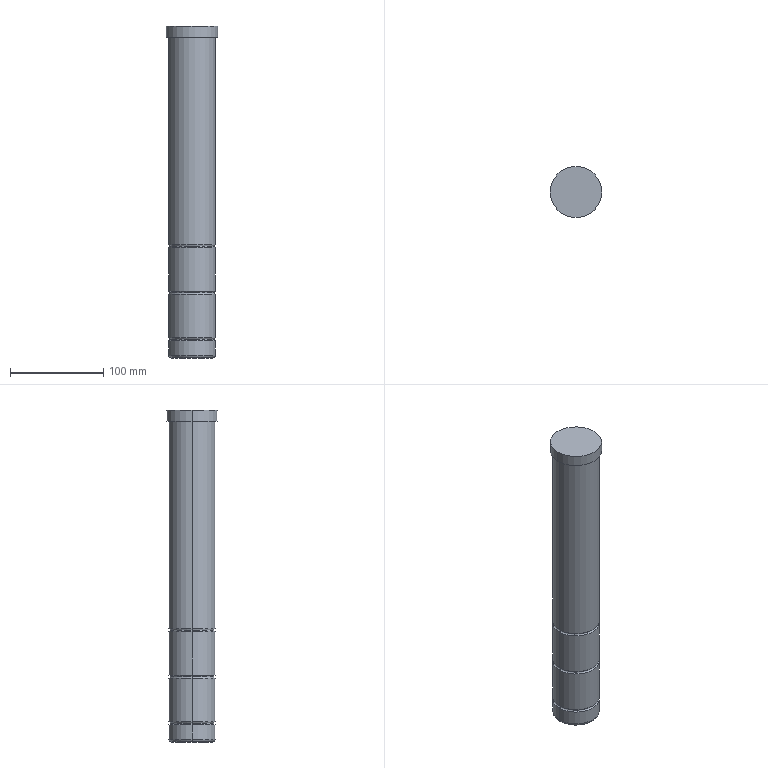Part | Creo | 1 solid | 29 faces | box 55 x 55 x 356 mm | volume 702034 mm3 | torus 16 | cylinder 10 | plane 3 | commonest cylinder face diameters 50 x8 55 x2
STEP:
#1=CARTESIAN_POINT('',(-272.,297.,-127.));
#2=VERTEX_POINT('',#1);
#3=CARTESIAN_POINT('',(-222.,297.,-127.));
#4=VERTEX_POINT('',#3);
#5=CARTESIAN_POINT('',(-247.,297.,-127.));
#6=DIRECTION('',(0.,0.,1.));
#7=DIRECTION('',(-1.,0.,0.));
#8=AXIS2_PLACEMENT_3D('',#5,#6,#7);
#9=CIRCLE('',#8,25.);
#10=EDGE_CURVE('',#2,#4,#9,.T.);
#11=ORIENTED_EDGE('',*,*,#10,.T.);
#12=CARTESIAN_POINT('',(-222.,297.,-142.5));
#13=VERTEX_POINT('',#12);
#14=CARTESIAN_POINT('',(-222.,297.,-127.));
#15=DIRECTION('',(0.,0.,-1.));
#16=VECTOR('',#15,15.5);
#17=LINE('',#14,#16);
#18=EDGE_CURVE('',#4,#13,#17,.T.);
#19=ORIENTED_EDGE('',*,*,#18,.T.);
#20=CARTESIAN_POINT('',(-272.,297.,-142.5));
#21=VERTEX_POINT('',#20);
#22=CARTESIAN_POINT('',(-247.,297.,-142.5));
#23=DIRECTION('',(0.,0.,-1.));
#24=DIRECTION('',(1.,0.,0.));
#25=AXIS2_PLACEMENT_3D('',#22,#23,#24);
#26=CIRCLE('',#25,25.);
#27=EDGE_CURVE('',#13,#21,#26,.T.);
#28=ORIENTED_EDGE('',*,*,#27,.T.);
#29=CARTESIAN_POINT('',(-272.,297.,-127.));
#30=DIRECTION('',(0.,0.,-1.));
#31=VECTOR('',#30,15.5);
#32=LINE('',#29,#31);
#33=EDGE_CURVE('',#2,#21,#32,.T.);
#34=ORIENTED_EDGE('',*,*,#33,.F.);
#35=EDGE_LOOP('',(#11,#19,#28,#34));
#36=FACE_OUTER_BOUND('',#35,.F.);
#37=CARTESIAN_POINT('',(-247.,297.,150.5));
#38=DIRECTION('',(0.,0.,-1.));
#39=DIRECTION('',(1.,0.,0.));
#40=AXIS2_PLACEMENT_3D('',#37,#38,#39);
#41=CYLINDRICAL_SURFACE('',#40,25.);
#42=ADVANCED_FACE('',(#36),#41,.T.);
#43=ORIENTED_EDGE('',*,*,#10,.F.);
#44=CARTESIAN_POINT('',(-270.5,297.,-125.5));
#45=VERTEX_POINT('',#44);
#46=CARTESIAN_POINT('',(-272.,297.,-125.5));
#47=DIRECTION('',(0.,-1.,0.));
#48=DIRECTION('',(0.,0.,-1.));
#49=AXIS2_PLACEMENT_3D('',#46,#47,#48);
#50=CIRCLE('',#49,1.5);
#51=EDGE_CURVE('',#2,#45,#50,.T.);
#52=ORIENTED_EDGE('',*,*,#51,.T.);
#53=CARTESIAN_POINT('',(-223.5,297.,-125.5));
#54=VERTEX_POINT('',#53);
#55=CARTESIAN_POINT('',(-247.,297.,-125.5));
#56=DIRECTION('',(0.,0.,-1.));
#57=DIRECTION('',(1.,0.,0.));
#58=AXIS2_PLACEMENT_3D('',#55,#56,#57);
#59=CIRCLE('',#58,23.5);
#60=EDGE_CURVE('',#54,#45,#59,.T.);
#61=ORIENTED_EDGE('',*,*,#60,.F.);
#62=CARTESIAN_POINT('',(-222.,297.,-125.5));
#63=DIRECTION('',(0.,1.,0.));
#64=DIRECTION('',(0.,0.,-1.));
#65=AXIS2_PLACEMENT_3D('',#62,#63,#64);
#66=CIRCLE('',#65,1.5);
#67=EDGE_CURVE('',#4,#54,#66,.T.);
#68=ORIENTED_EDGE('',*,*,#67,.F.);
#69=EDGE_LOOP('',(#43,#52,#61,#68));
#70=FACE_OUTER_BOUND('',#69,.F.);
#71=CARTESIAN_POINT('',(-247.,297.,-125.5));
#72=DIRECTION('',(0.,0.,-1.));
#73=DIRECTION('',(1.,0.,0.));
#74=AXIS2_PLACEMENT_3D('',#71,#72,#73);
#75=TOROIDAL_SURFACE('',#74,25.,1.5);
#76=ADVANCED_FACE('',(#70),#75,.F.);
#77=CARTESIAN_POINT('',(-247.,297.,-127.));
#78=DIRECTION('',(0.,0.,1.));
#79=DIRECTION('',(1.,0.,0.));
#80=AXIS2_PLACEMENT_3D('',#77,#78,#79);
#81=CIRCLE('',#80,25.);
#82=EDGE_CURVE('',#4,#2,#81,.T.);
#83=ORIENTED_EDGE('',*,*,#82,.F.);
#84=ORIENTED_EDGE('',*,*,#67,.T.);
#85=CARTESIAN_POINT('',(-247.,297.,-125.5));
#86=DIRECTION('',(0.,0.,-1.));
#87=DIRECTION('',(-1.,0.,0.));
#88=AXIS2_PLACEMENT_3D('',#85,#86,#87);
#89=CIRCLE('',#88,23.5);
#90=EDGE_CURVE('',#45,#54,#89,.T.);
#91=ORIENTED_EDGE('',*,*,#90,.F.);
#92=ORIENTED_EDGE('',*,*,#51,.F.);
#93=EDGE_LOOP('',(#83,#84,#91,#92));
#94=FACE_OUTER_BOUND('',#93,.F.);
#95=CARTESIAN_POINT('',(-247.,297.,-125.5));
#96=DIRECTION('',(0.,0.,-1.));
#97=DIRECTION('',(1.,0.,0.));
#98=AXIS2_PLACEMENT_3D('',#95,#96,#97);
#99=TOROIDAL_SURFACE('',#98,25.,1.5);
#100=ADVANCED_FACE('',(#94),#99,.F.);
#101=ORIENTED_EDGE('',*,*,#82,.T.);
#102=ORIENTED_EDGE('',*,*,#33,.T.);
#103=CARTESIAN_POINT('',(-247.,297.,-142.5));
#104=DIRECTION('',(0.,0.,-1.));
#105=DIRECTION('',(-1.,0.,0.));
#106=AXIS2_PLACEMENT_3D('',#103,#104,#105);
#107=CIRCLE('',#106,25.);
#108=EDGE_CURVE('',#21,#13,#107,.T.);
#109=ORIENTED_EDGE('',*,*,#108,.T.);
#110=ORIENTED_EDGE('',*,*,#18,.F.);
#111=EDGE_LOOP('',(#101,#102,#109,#110));
#112=FACE_OUTER_BOUND('',#111,.F.);
#113=CARTESIAN_POINT('',(-247.,297.,150.5));
#114=DIRECTION('',(0.,0.,-1.));
#115=DIRECTION('',(1.,0.,0.));
#116=AXIS2_PLACEMENT_3D('',#113,#114,#115);
#117=CYLINDRICAL_SURFACE('',#116,25.);
#118=ADVANCED_FACE('',(#112),#117,.T.);
#119=ORIENTED_EDGE('',*,*,#108,.F.);
#120=CARTESIAN_POINT('',(-271.121,297.,-144.621));
#121=VERTEX_POINT('',#120);
#122=CARTESIAN_POINT('',(-269.,297.,-142.5));
#123=DIRECTION('',(0.,-1.,0.));
#124=DIRECTION('',(-1.,0.,0.));
#125=AXIS2_PLACEMENT_3D('',#122,#123,#124);
#126=CIRCLE('',#125,3.);
#127=EDGE_CURVE('',#21,#121,#126,.T.);
#128=ORIENTED_EDGE('',*,*,#127,.T.);
#129=CARTESIAN_POINT('',(-222.879,297.,-144.621));
#130=VERTEX_POINT('',#129);
#131=CARTESIAN_POINT('',(-247.,297.,-144.621));
#132=DIRECTION('',(0.,0.,-1.));
#133=DIRECTION('',(-1.,0.,0.));
#134=AXIS2_PLACEMENT_3D('',#131,#132,#133);
#135=CIRCLE('',#134,24.121);
#136=EDGE_CURVE('',#121,#130,#135,.T.);
#137=ORIENTED_EDGE('',*,*,#136,.T.);
#138=CARTESIAN_POINT('',(-225.,297.,-142.5));
#139=DIRECTION('',(0.,1.,0.));
#140=DIRECTION('',(1.,0.,0.));
#141=AXIS2_PLACEMENT_3D('',#138,#139,#140);
#142=CIRCLE('',#141,3.);
#143=EDGE_CURVE('',#13,#130,#142,.T.);
#144=ORIENTED_EDGE('',*,*,#143,.F.);
#145=EDGE_LOOP('',(#119,#128,#137,#144));
#146=FACE_OUTER_BOUND('',#145,.F.);
#147=CARTESIAN_POINT('',(-247.,297.,-142.5));
#148=DIRECTION('',(0.,0.,-1.));
#149=DIRECTION('',(1.,0.,0.));
#150=AXIS2_PLACEMENT_3D('',#147,#148,#149);
#151=TOROIDAL_SURFACE('',#150,22.,3.);
#152=ADVANCED_FACE('',(#146),#151,.T.);
#153=ORIENTED_EDGE('',*,*,#27,.F.);
#154=ORIENTED_EDGE('',*,*,#143,.T.);
#155=CARTESIAN_POINT('',(-247.,297.,-144.621));
#156=DIRECTION('',(0.,0.,-1.));
#157=DIRECTION('',(1.,0.,0.));
#158=AXIS2_PLACEMENT_3D('',#155,#156,#157);
#159=CIRCLE('',#158,24.121);
#160=EDGE_CURVE('',#130,#121,#159,.T.);
#161=ORIENTED_EDGE('',*,*,#160,.T.);
#162=ORIENTED_EDGE('',*,*,#127,.F.);
#163=EDGE_LOOP('',(#153,#154,#161,#162));
#164=FACE_OUTER_BOUND('',#163,.F.);
#165=CARTESIAN_POINT('',(-247.,297.,-142.5));
#166=DIRECTION('',(0.,0.,-1.));
#167=DIRECTION('',(1.,0.,0.));
#168=AXIS2_PLACEMENT_3D('',#165,#166,#167);
#169=TOROIDAL_SURFACE('',#168,22.,3.);
#170=ADVANCED_FACE('',(#164),#169,.T.);
#171=CARTESIAN_POINT('',(-225.,297.,-145.5));
#172=VERTEX_POINT('',#171);
#173=CARTESIAN_POINT('',(-269.,297.,-145.5));
#174=VERTEX_POINT('',#173);
#175=CARTESIAN_POINT('',(-247.,297.,-145.5));
#176=DIRECTION('',(0.,0.,-1.));
#177=DIRECTION('',(1.,0.,0.));
#178=AXIS2_PLACEMENT_3D('',#175,#176,#177);
#179=CIRCLE('',#178,22.);
#180=EDGE_CURVE('',#172,#174,#179,.T.);
#181=ORIENTED_EDGE('',*,*,#180,.T.);
#182=CARTESIAN_POINT('',(-269.,297.,-142.5));
#183=DIRECTION('',(0.,-1.,0.));
#184=DIRECTION('',(-0.7071,0.,-0.7071));
#185=AXIS2_PLACEMENT_3D('',#182,#183,#184);
#186=CIRCLE('',#185,3.);
#187=EDGE_CURVE('',#121,#174,#186,.T.);
#188=ORIENTED_EDGE('',*,*,#187,.F.);
#189=ORIENTED_EDGE('',*,*,#160,.F.);
#190=CARTESIAN_POINT('',(-225.,297.,-142.5));
#191=DIRECTION('',(0.,1.,0.));
#192=DIRECTION('',(0.7071,0.,-0.7071));
#193=AXIS2_PLACEMENT_3D('',#190,#191,#192);
#194=CIRCLE('',#193,3.);
#195=EDGE_CURVE('',#130,#172,#194,.T.);
#196=ORIENTED_EDGE('',*,*,#195,.T.);
#197=EDGE_LOOP('',(#181,#188,#189,#196));
#198=FACE_OUTER_BOUND('',#197,.F.);
#199=CARTESIAN_POINT('',(-247.,297.,-142.5));
#200=DIRECTION('',(0.,0.,-1.));
#201=DIRECTION('',(1.,0.,0.));
#202=AXIS2_PLACEMENT_3D('',#199,#200,#201);
#203=TOROIDAL_SURFACE('',#202,22.,3.);
#204=ADVANCED_FACE('',(#198),#203,.T.);
#205=ORIENTED_EDGE('',*,*,#180,.F.);
#206=CARTESIAN_POINT('',(-247.,297.,-145.5));
#207=DIRECTION('',(0.,0.,-1.));
#208=DIRECTION('',(-1.,0.,0.));
#209=AXIS2_PLACEMENT_3D('',#206,#207,#208);
#210=CIRCLE('',#209,22.);
#211=EDGE_CURVE('',#174,#172,#210,.T.);
#212=ORIENTED_EDGE('',*,*,#211,.F.);
#213=EDGE_LOOP('',(#205,#212));
#214=FACE_OUTER_BOUND('',#213,.F.);
#215=CARTESIAN_POINT('',(-247.,297.,-145.5));
#216=DIRECTION('',(0.,0.,-1.));
#217=DIRECTION('',(1.,0.,0.));
#218=AXIS2_PLACEMENT_3D('',#215,#216,#217);
#219=PLANE('',#218);
#220=ADVANCED_FACE('',(#214),#219,.T.);
#221=ORIENTED_EDGE('',*,*,#211,.T.);
#222=ORIENTED_EDGE('',*,*,#195,.F.);
#223=ORIENTED_EDGE('',*,*,#136,.F.);
#224=ORIENTED_EDGE('',*,*,#187,.T.);
#225=EDGE_LOOP('',(#221,#222,#223,#224));
#226=FACE_OUTER_BOUND('',#225,.F.);
#227=CARTESIAN_POINT('',(-247.,297.,-142.5));
#228=DIRECTION('',(0.,0.,-1.));
#229=DIRECTION('',(1.,0.,0.));
#230=AXIS2_PLACEMENT_3D('',#227,#228,#229);
#231=TOROIDAL_SURFACE('',#230,22.,3.);
#232=ADVANCED_FACE('',(#226),#231,.T.);
#233=CARTESIAN_POINT('',(-272.,297.,-124.));
#234=VERTEX_POINT('',#233);
#235=CARTESIAN_POINT('',(-222.,297.,-124.));
#236=VERTEX_POINT('',#235);
#237=CARTESIAN_POINT('',(-247.,297.,-124.));
#238=DIRECTION('',(0.,0.,-1.));
#239=DIRECTION('',(-1.,0.,0.));
#240=AXIS2_PLACEMENT_3D('',#237,#238,#239);
#241=CIRCLE('',#240,25.);
#242=EDGE_CURVE('',#234,#236,#241,.T.);
#243=ORIENTED_EDGE('',*,*,#242,.F.);
#244=CARTESIAN_POINT('',(-272.,297.,-125.5));
#245=DIRECTION('',(0.,-1.,0.));
#246=DIRECTION('',(1.,0.,0.));
#247=AXIS2_PLACEMENT_3D('',#244,#245,#246);
#248=CIRCLE('',#247,1.5);
#249=EDGE_CURVE('',#45,#234,#248,.T.);
#250=ORIENTED_EDGE('',*,*,#249,.F.);
#251=ORIENTED_EDGE('',*,*,#90,.T.);
#252=CARTESIAN_POINT('',(-222.,297.,-125.5));
#253=DIRECTION('',(0.,1.,0.));
#254=DIRECTION('',(-1.,0.,0.));
#255=AXIS2_PLACEMENT_3D('',#252,#253,#254);
#256=CIRCLE('',#255,1.5);
#257=EDGE_CURVE('',#54,#236,#256,.T.);
#258=ORIENTED_EDGE('',*,*,#257,.T.);
#259=EDGE_LOOP('',(#243,#250,#251,#258));
#260=FACE_OUTER_BOUND('',#259,.F.);
#261=CARTESIAN_POINT('',(-247.,297.,-125.5));
#262=DIRECTION('',(0.,0.,-1.));
#263=DIRECTION('',(1.,0.,0.));
#264=AXIS2_PLACEMENT_3D('',#261,#262,#263);
#265=TOROIDAL_SURFACE('',#264,25.,1.5);
#266=ADVANCED_FACE('',(#260),#265,.F.);
#267=ORIENTED_EDGE('',*,*,#242,.T.);
#268=CARTESIAN_POINT('',(-222.,297.,-77.));
#269=VERTEX_POINT('',#268);
#270=CARTESIAN_POINT('',(-222.,297.,-77.));
#271=DIRECTION('',(0.,0.,-1.));
#272=VECTOR('',#271,47.);
#273=LINE('',#270,#272);
#274=EDGE_CURVE('',#269,#236,#273,.T.);
#275=ORIENTED_EDGE('',*,*,#274,.F.);
#276=CARTESIAN_POINT('',(-272.,297.,-77.));
#277=VERTEX_POINT('',#276);
#278=CARTESIAN_POINT('',(-247.,297.,-77.));
#279=DIRECTION('',(0.,0.,1.));
#280=DIRECTION('',(1.,0.,0.));
#281=AXIS2_PLACEMENT_3D('',#278,#279,#280);
#282=CIRCLE('',#281,25.);
#283=EDGE_CURVE('',#269,#277,#282,.T.);
#284=ORIENTED_EDGE('',*,*,#283,.T.);
#285=CARTESIAN_POINT('',(-272.,297.,-77.));
#286=DIRECTION('',(0.,0.,-1.));
#287=VECTOR('',#286,47.);
#288=LINE('',#285,#287);
#289=EDGE_CURVE('',#277,#234,#288,.T.);
#290=ORIENTED_EDGE('',*,*,#289,.T.);
#291=EDGE_LOOP('',(#267,#275,#284,#290));
#292=FACE_OUTER_BOUND('',#291,.F.);
#293=CARTESIAN_POINT('',(-247.,297.,150.5));
#294=DIRECTION('',(0.,0.,-1.));
#295=DIRECTION('',(1.,0.,0.));
#296=AXIS2_PLACEMENT_3D('',#293,#294,#295);
#297=CYLINDRICAL_SURFACE('',#296,25.);
#298=ADVANCED_FACE('',(#292),#297,.T.);
#299=CARTESIAN_POINT('',(-247.,297.,-124.));
#300=DIRECTION('',(0.,0.,-1.));
#301=DIRECTION('',(1.,0.,0.));
#302=AXIS2_PLACEMENT_3D('',#299,#300,#301);
#303=CIRCLE('',#302,25.);
#304=EDGE_CURVE('',#236,#234,#303,.T.);
#305=ORIENTED_EDGE('',*,*,#304,.T.);
#306=ORIENTED_EDGE('',*,*,#289,.F.);
#307=CARTESIAN_POINT('',(-247.,297.,-77.));
#308=DIRECTION('',(0.,0.,1.));
#309=DIRECTION('',(-1.,0.,0.));
#310=AXIS2_PLACEMENT_3D('',#307,#308,#309);
#311=CIRCLE('',#310,25.);
#312=EDGE_CURVE('',#277,#269,#311,.T.);
#313=ORIENTED_EDGE('',*,*,#312,.T.);
#314=ORIENTED_EDGE('',*,*,#274,.T.);
#315=EDGE_LOOP('',(#305,#306,#313,#314));
#316=FACE_OUTER_BOUND('',#315,.F.);
#317=CARTESIAN_POINT('',(-247.,297.,150.5));
#318=DIRECTION('',(0.,0.,-1.));
#319=DIRECTION('',(1.,0.,0.));
#320=AXIS2_PLACEMENT_3D('',#317,#318,#319);
#321=CYLINDRICAL_SURFACE('',#320,25.);
#322=ADVANCED_FACE('',(#316),#321,.T.);
#323=ORIENTED_EDGE('',*,*,#304,.F.);
#324=ORIENTED_EDGE('',*,*,#257,.F.);
#325=ORIENTED_EDGE('',*,*,#60,.T.);
#326=ORIENTED_EDGE('',*,*,#249,.T.);
#327=EDGE_LOOP('',(#323,#324,#325,#326));
#328=FACE_OUTER_BOUND('',#327,.F.);
#329=CARTESIAN_POINT('',(-247.,297.,-125.5));
#330=DIRECTION('',(0.,0.,-1.));
#331=DIRECTION('',(1.,0.,0.));
#332=AXIS2_PLACEMENT_3D('',#329,#330,#331);
#333=TOROIDAL_SURFACE('',#332,25.,1.5);
#334=ADVANCED_FACE('',(#328),#333,.F.);
#335=ORIENTED_EDGE('',*,*,#312,.F.);
#336=CARTESIAN_POINT('',(-270.5,297.,-75.5));
#337=VERTEX_POINT('',#336);
#338=CARTESIAN_POINT('',(-272.,297.,-75.5));
#339=DIRECTION('',(0.,-1.,0.));
#340=DIRECTION('',(0.,0.,-1.));
#341=AXIS2_PLACEMENT_3D('',#338,#339,#340);
#342=CIRCLE('',#341,1.5);
#343=EDGE_CURVE('',#277,#337,#342,.T.);
#344=ORIENTED_EDGE('',*,*,#343,.T.);
#345=CARTESIAN_POINT('',(-223.5,297.,-75.5));
#346=VERTEX_POINT('',#345);
#347=CARTESIAN_POINT('',(-247.,297.,-75.5));
#348=DIRECTION('',(0.,0.,-1.));
#349=DIRECTION('',(1.,0.,0.));
#350=AXIS2_PLACEMENT_3D('',#347,#348,#349);
#351=CIRCLE('',#350,23.5);
#352=EDGE_CURVE('',#346,#337,#351,.T.);
#353=ORIENTED_EDGE('',*,*,#352,.F.);
#354=CARTESIAN_POINT('',(-222.,297.,-75.5));
#355=DIRECTION('',(0.,1.,0.));
#356=DIRECTION('',(0.,0.,-1.));
#357=AXIS2_PLACEMENT_3D('',#354,#355,#356);
#358=CIRCLE('',#357,1.5);
#359=EDGE_CURVE('',#269,#346,#358,.T.);
#360=ORIENTED_EDGE('',*,*,#359,.F.);
#361=EDGE_LOOP('',(#335,#344,#353,#360));
#362=FACE_OUTER_BOUND('',#361,.F.);
#363=CARTESIAN_POINT('',(-247.,297.,-75.5));
#364=DIRECTION('',(0.,0.,-1.));
#365=DIRECTION('',(1.,0.,0.));
#366=AXIS2_PLACEMENT_3D('',#363,#364,#365);
#367=TOROIDAL_SURFACE('',#366,25.,1.5);
#368=ADVANCED_FACE('',(#362),#367,.F.);
#369=ORIENTED_EDGE('',*,*,#283,.F.);
#370=ORIENTED_EDGE('',*,*,#359,.T.);
#371=CARTESIAN_POINT('',(-247.,297.,-75.5));
#372=DIRECTION('',(0.,0.,-1.));
#373=DIRECTION('',(-1.,0.,0.));
#374=AXIS2_PLACEMENT_3D('',#371,#372,#373);
#375=CIRCLE('',#374,23.5);
#376=EDGE_CURVE('',#337,#346,#375,.T.);
#377=ORIENTED_EDGE('',*,*,#376,.F.);
#378=ORIENTED_EDGE('',*,*,#343,.F.);
#379=EDGE_LOOP('',(#369,#370,#377,#378));
#380=FACE_OUTER_BOUND('',#379,.F.);
#381=CARTESIAN_POINT('',(-247.,297.,-75.5));
#382=DIRECTION('',(0.,0.,-1.));
#383=DIRECTION('',(1.,0.,0.));
#384=AXIS2_PLACEMENT_3D('',#381,#382,#383);
#385=TOROIDAL_SURFACE('',#384,25.,1.5);
#386=ADVANCED_FACE('',(#380),#385,.F.);
#387=CARTESIAN_POINT('',(-272.,297.,-74.));
#388=VERTEX_POINT('',#387);
#389=CARTESIAN_POINT('',(-222.,297.,-74.));
#390=VERTEX_POINT('',#389);
#391=CARTESIAN_POINT('',(-247.,297.,-74.));
#392=DIRECTION('',(0.,0.,-1.));
#393=DIRECTION('',(-1.,0.,0.));
#394=AXIS2_PLACEMENT_3D('',#391,#392,#393);
#395=CIRCLE('',#394,25.);
#396=EDGE_CURVE('',#388,#390,#395,.T.);
#397=ORIENTED_EDGE('',*,*,#396,.F.);
#398=CARTESIAN_POINT('',(-272.,297.,-75.5));
#399=DIRECTION('',(0.,-1.,0.));
#400=DIRECTION('',(1.,0.,0.));
#401=AXIS2_PLACEMENT_3D('',#398,#399,#400);
#402=CIRCLE('',#401,1.5);
#403=EDGE_CURVE('',#337,#388,#402,.T.);
#404=ORIENTED_EDGE('',*,*,#403,.F.);
#405=ORIENTED_EDGE('',*,*,#376,.T.);
#406=CARTESIAN_POINT('',(-222.,297.,-75.5));
#407=DIRECTION('',(0.,1.,0.));
#408=DIRECTION('',(-1.,0.,0.));
#409=AXIS2_PLACEMENT_3D('',#406,#407,#408);
#410=CIRCLE('',#409,1.5);
#411=EDGE_CURVE('',#346,#390,#410,.T.);
#412=ORIENTED_EDGE('',*,*,#411,.T.);
#413=EDGE_LOOP('',(#397,#404,#405,#412));
#414=FACE_OUTER_BOUND('',#413,.F.);
#415=CARTESIAN_POINT('',(-247.,297.,-75.5));
#416=DIRECTION('',(0.,0.,-1.));
#417=DIRECTION('',(1.,0.,0.));
#418=AXIS2_PLACEMENT_3D('',#415,#416,#417);
#419=TOROIDAL_SURFACE('',#418,25.,1.5);
#420=ADVANCED_FACE('',(#414),#419,.F.);
#421=ORIENTED_EDGE('',*,*,#396,.T.);
#422=CARTESIAN_POINT('',(-222.,297.,-27.));
#423=VERTEX_POINT('',#422);
#424=CARTESIAN_POINT('',(-222.,297.,-27.));
#425=DIRECTION('',(0.,0.,-1.));
#426=VECTOR('',#425,47.);
#427=LINE('',#424,#426);
#428=EDGE_CURVE('',#423,#390,#427,.T.);
#429=ORIENTED_EDGE('',*,*,#428,.F.);
#430=CARTESIAN_POINT('',(-272.,297.,-27.));
#431=VERTEX_POINT('',#430);
#432=CARTESIAN_POINT('',(-247.,297.,-27.));
#433=DIRECTION('',(0.,0.,1.));
#434=DIRECTION('',(1.,0.,0.));
#435=AXIS2_PLACEMENT_3D('',#432,#433,#434);
#436=CIRCLE('',#435,25.);
#437=EDGE_CURVE('',#423,#431,#436,.T.);
#438=ORIENTED_EDGE('',*,*,#437,.T.);
#439=CARTESIAN_POINT('',(-272.,297.,-27.));
#440=DIRECTION('',(0.,0.,-1.));
#441=VECTOR('',#440,47.);
#442=LINE('',#439,#441);
#443=EDGE_CURVE('',#431,#388,#442,.T.);
#444=ORIENTED_EDGE('',*,*,#443,.T.);
#445=EDGE_LOOP('',(#421,#429,#438,#444));
#446=FACE_OUTER_BOUND('',#445,.F.);
#447=CARTESIAN_POINT('',(-247.,297.,150.5));
#448=DIRECTION('',(0.,0.,-1.));
#449=DIRECTION('',(1.,0.,0.));
#450=AXIS2_PLACEMENT_3D('',#447,#448,#449);
#451=CYLINDRICAL_SURFACE('',#450,25.);
#452=ADVANCED_FACE('',(#446),#451,.T.);
#453=CARTESIAN_POINT('',(-247.,297.,-74.));
#454=DIRECTION('',(0.,0.,-1.));
#455=DIRECTION('',(1.,0.,0.));
#456=AXIS2_PLACEMENT_3D('',#453,#454,#455);
#457=CIRCLE('',#456,25.);
#458=EDGE_CURVE('',#390,#388,#457,.T.);
#459=ORIENTED_EDGE('',*,*,#458,.T.);
#460=ORIENTED_EDGE('',*,*,#443,.F.);
#461=CARTESIAN_POINT('',(-247.,297.,-27.));
#462=DIRECTION('',(0.,0.,1.));
#463=DIRECTION('',(-1.,0.,0.));
#464=AXIS2_PLACEMENT_3D('',#461,#462,#463);
#465=CIRCLE('',#464,25.);
#466=EDGE_CURVE('',#431,#423,#465,.T.);
#467=ORIENTED_EDGE('',*,*,#466,.T.);
#468=ORIENTED_EDGE('',*,*,#428,.T.);
#469=EDGE_LOOP('',(#459,#460,#467,#468));
#470=FACE_OUTER_BOUND('',#469,.F.);
#471=CARTESIAN_POINT('',(-247.,297.,150.5));
#472=DIRECTION('',(0.,0.,-1.));
#473=DIRECTION('',(1.,0.,0.));
#474=AXIS2_PLACEMENT_3D('',#471,#472,#473);
#475=CYLINDRICAL_SURFACE('',#474,25.);
#476=ADVANCED_FACE('',(#470),#475,.T.);
#477=ORIENTED_EDGE('',*,*,#458,.F.);
#478=ORIENTED_EDGE('',*,*,#411,.F.);
#479=ORIENTED_EDGE('',*,*,#352,.T.);
#480=ORIENTED_EDGE('',*,*,#403,.T.);
#481=EDGE_LOOP('',(#477,#478,#479,#480));
#482=FACE_OUTER_BOUND('',#481,.F.);
#483=CARTESIAN_POINT('',(-247.,297.,-75.5));
#484=DIRECTION('',(0.,0.,-1.));
#485=DIRECTION('',(1.,0.,0.));
#486=AXIS2_PLACEMENT_3D('',#483,#484,#485);
#487=TOROIDAL_SURFACE('',#486,25.,1.5);
#488=ADVANCED_FACE('',(#482),#487,.F.);
#489=ORIENTED_EDGE('',*,*,#466,.F.);
#490=CARTESIAN_POINT('',(-270.5,297.,-25.5));
#491=VERTEX_POINT('',#490);
#492=CARTESIAN_POINT('',(-272.,297.,-25.5));
#493=DIRECTION('',(0.,-1.,0.));
#494=DIRECTION('',(0.,0.,-1.));
#495=AXIS2_PLACEMENT_3D('',#492,#493,#494);
#496=CIRCLE('',#495,1.5);
#497=EDGE_CURVE('',#431,#491,#496,.T.);
#498=ORIENTED_EDGE('',*,*,#497,.T.);
#499=CARTESIAN_POINT('',(-223.5,297.,-25.5));
#500=VERTEX_POINT('',#499);
#501=CARTESIAN_POINT('',(-247.,297.,-25.5));
#502=DIRECTION('',(0.,0.,-1.));
#503=DIRECTION('',(1.,0.,0.));
#504=AXIS2_PLACEMENT_3D('',#501,#502,#503);
#505=CIRCLE('',#504,23.5);
#506=EDGE_CURVE('',#500,#491,#505,.T.);
#507=ORIENTED_EDGE('',*,*,#506,.F.);
#508=CARTESIAN_POINT('',(-222.,297.,-25.5));
#509=DIRECTION('',(0.,1.,0.));
#510=DIRECTION('',(0.,0.,-1.));
#511=AXIS2_PLACEMENT_3D('',#508,#509,#510);
#512=CIRCLE('',#511,1.5);
#513=EDGE_CURVE('',#423,#500,#512,.T.);
#514=ORIENTED_EDGE('',*,*,#513,.F.);
#515=EDGE_LOOP('',(#489,#498,#507,#514));
#516=FACE_OUTER_BOUND('',#515,.F.);
#517=CARTESIAN_POINT('',(-247.,297.,-25.5));
#518=DIRECTION('',(0.,0.,-1.));
#519=DIRECTION('',(1.,0.,0.));
#520=AXIS2_PLACEMENT_3D('',#517,#518,#519);
#521=TOROIDAL_SURFACE('',#520,25.,1.5);
#522=ADVANCED_FACE('',(#516),#521,.F.);
#523=ORIENTED_EDGE('',*,*,#437,.F.);
#524=ORIENTED_EDGE('',*,*,#513,.T.);
#525=CARTESIAN_POINT('',(-247.,297.,-25.5));
#526=DIRECTION('',(0.,0.,-1.));
#527=DIRECTION('',(-1.,0.,0.));
#528=AXIS2_PLACEMENT_3D('',#525,#526,#527);
#529=CIRCLE('',#528,23.5);
#530=EDGE_CURVE('',#491,#500,#529,.T.);
#531=ORIENTED_EDGE('',*,*,#530,.F.);
#532=ORIENTED_EDGE('',*,*,#497,.F.);
#533=EDGE_LOOP('',(#523,#524,#531,#532));
#534=FACE_OUTER_BOUND('',#533,.F.);
#535=CARTESIAN_POINT('',(-247.,297.,-25.5));
#536=DIRECTION('',(0.,0.,-1.));
#537=DIRECTION('',(1.,0.,0.));
#538=AXIS2_PLACEMENT_3D('',#535,#536,#537);
#539=TOROIDAL_SURFACE('',#538,25.,1.5);
#540=ADVANCED_FACE('',(#534),#539,.F.);
#541=CARTESIAN_POINT('',(-272.,297.,-24.));
#542=VERTEX_POINT('',#541);
#543=CARTESIAN_POINT('',(-222.,297.,-24.));
#544=VERTEX_POINT('',#543);
#545=CARTESIAN_POINT('',(-247.,297.,-24.));
#546=DIRECTION('',(0.,0.,-1.));
#547=DIRECTION('',(-1.,0.,0.));
#548=AXIS2_PLACEMENT_3D('',#545,#546,#547);
#549=CIRCLE('',#548,25.);
#550=EDGE_CURVE('',#542,#544,#549,.T.);
#551=ORIENTED_EDGE('',*,*,#550,.F.);
#552=CARTESIAN_POINT('',(-272.,297.,-25.5));
#553=DIRECTION('',(0.,-1.,0.));
#554=DIRECTION('',(1.,0.,0.));
#555=AXIS2_PLACEMENT_3D('',#552,#553,#554);
#556=CIRCLE('',#555,1.5);
#557=EDGE_CURVE('',#491,#542,#556,.T.);
#558=ORIENTED_EDGE('',*,*,#557,.F.);
#559=ORIENTED_EDGE('',*,*,#530,.T.);
#560=CARTESIAN_POINT('',(-222.,297.,-25.5));
#561=DIRECTION('',(0.,1.,0.));
#562=DIRECTION('',(-1.,0.,0.));
#563=AXIS2_PLACEMENT_3D('',#560,#561,#562);
#564=CIRCLE('',#563,1.5);
#565=EDGE_CURVE('',#500,#544,#564,.T.);
#566=ORIENTED_EDGE('',*,*,#565,.T.);
#567=EDGE_LOOP('',(#551,#558,#559,#566));
#568=FACE_OUTER_BOUND('',#567,.F.);
#569=CARTESIAN_POINT('',(-247.,297.,-25.5));
#570=DIRECTION('',(0.,0.,-1.));
#571=DIRECTION('',(1.,0.,0.));
#572=AXIS2_PLACEMENT_3D('',#569,#570,#571);
#573=TOROIDAL_SURFACE('',#572,25.,1.5);
#574=ADVANCED_FACE('',(#568),#573,.F.);
#575=CARTESIAN_POINT('',(-222.,297.,198.5));
#576=VERTEX_POINT('',#575);
#577=CARTESIAN_POINT('',(-272.,297.,198.5));
#578=VERTEX_POINT('',#577);
#579=CARTESIAN_POINT('',(-247.,297.,198.5));
#580=DIRECTION('',(0.,0.,1.));
#581=DIRECTION('',(1.,0.,0.));
#582=AXIS2_PLACEMENT_3D('',#579,#580,#581);
#583=CIRCLE('',#582,25.);
#584=EDGE_CURVE('',#576,#578,#583,.T.);
#585=ORIENTED_EDGE('',*,*,#584,.T.);
#586=CARTESIAN_POINT('',(-272.,297.,198.5));
#587=DIRECTION('',(0.,0.,-1.));
#588=VECTOR('',#587,222.5);
#589=LINE('',#586,#588);
#590=EDGE_CURVE('',#578,#542,#589,.T.);
#591=ORIENTED_EDGE('',*,*,#590,.T.);
#592=ORIENTED_EDGE('',*,*,#550,.T.);
#593=CARTESIAN_POINT('',(-222.,297.,198.5));
#594=DIRECTION('',(0.,0.,-1.));
#595=VECTOR('',#594,222.5);
#596=LINE('',#593,#595);
#597=EDGE_CURVE('',#576,#544,#596,.T.);
#598=ORIENTED_EDGE('',*,*,#597,.F.);
#599=EDGE_LOOP('',(#585,#591,#592,#598));
#600=FACE_OUTER_BOUND('',#599,.F.);
#601=CARTESIAN_POINT('',(-247.,297.,150.5));
#602=DIRECTION('',(0.,0.,-1.));
#603=DIRECTION('',(1.,0.,0.));
#604=AXIS2_PLACEMENT_3D('',#601,#602,#603);
#605=CYLINDRICAL_SURFACE('',#604,25.);
#606=ADVANCED_FACE('',(#600),#605,.T.);
#607=CARTESIAN_POINT('',(-274.5,297.,198.5));
#608=VERTEX_POINT('',#607);
#609=CARTESIAN_POINT('',(-219.5,297.,198.5));
#610=VERTEX_POINT('',#609);
#611=CARTESIAN_POINT('',(-247.,297.,198.5));
#612=DIRECTION('',(0.,0.,-1.));
#613=DIRECTION('',(-1.,0.,0.));
#614=AXIS2_PLACEMENT_3D('',#611,#612,#613);
#615=CIRCLE('',#614,27.5);
#616=EDGE_CURVE('',#608,#610,#615,.T.);
#617=ORIENTED_EDGE('',*,*,#616,.F.);
#618=CARTESIAN_POINT('',(-247.,297.,198.5));
#619=DIRECTION('',(0.,0.,-1.));
#620=DIRECTION('',(1.,0.,0.));
#621=AXIS2_PLACEMENT_3D('',#618,#619,#620);
#622=CIRCLE('',#621,27.5);
#623=EDGE_CURVE('',#610,#608,#622,.T.);
#624=ORIENTED_EDGE('',*,*,#623,.F.);
#625=EDGE_LOOP('',(#617,#624));
#626=FACE_OUTER_BOUND('',#625,.F.);
#627=ORIENTED_EDGE('',*,*,#584,.F.);
#628=CARTESIAN_POINT('',(-247.,297.,198.5));
#629=DIRECTION('',(0.,0.,1.));
#630=DIRECTION('',(-1.,0.,0.));
#631=AXIS2_PLACEMENT_3D('',#628,#629,#630);
#632=CIRCLE('',#631,25.);
#633=EDGE_CURVE('',#578,#576,#632,.T.);
#634=ORIENTED_EDGE('',*,*,#633,.F.);
#635=EDGE_LOOP('',(#627,#634));
#636=FACE_BOUND('',#635,.F.);
#637=CARTESIAN_POINT('',(-247.,297.,198.5));
#638=DIRECTION('',(0.,0.,-1.));
#639=DIRECTION('',(1.,0.,0.));
#640=AXIS2_PLACEMENT_3D('',#637,#638,#639);
#641=PLANE('',#640);
#642=ADVANCED_FACE('',(#626,#636),#641,.T.);
#643=ORIENTED_EDGE('',*,*,#633,.T.);
#644=ORIENTED_EDGE('',*,*,#597,.T.);
#645=CARTESIAN_POINT('',(-247.,297.,-24.));
#646=DIRECTION('',(0.,0.,-1.));
#647=DIRECTION('',(1.,0.,0.));
#648=AXIS2_PLACEMENT_3D('',#645,#646,#647);
#649=CIRCLE('',#648,25.);
#650=EDGE_CURVE('',#544,#542,#649,.T.);
#651=ORIENTED_EDGE('',*,*,#650,.T.);
#652=ORIENTED_EDGE('',*,*,#590,.F.);
#653=EDGE_LOOP('',(#643,#644,#651,#652));
#654=FACE_OUTER_BOUND('',#653,.F.);
#655=CARTESIAN_POINT('',(-247.,297.,150.5));
#656=DIRECTION('',(0.,0.,-1.));
#657=DIRECTION('',(1.,0.,0.));
#658=AXIS2_PLACEMENT_3D('',#655,#656,#657);
#659=CYLINDRICAL_SURFACE('',#658,25.);
#660=ADVANCED_FACE('',(#654),#659,.T.);
#661=ORIENTED_EDGE('',*,*,#650,.F.);
#662=ORIENTED_EDGE('',*,*,#565,.F.);
#663=ORIENTED_EDGE('',*,*,#506,.T.);
#664=ORIENTED_EDGE('',*,*,#557,.T.);
#665=EDGE_LOOP('',(#661,#662,#663,#664));
#666=FACE_OUTER_BOUND('',#665,.F.);
#667=CARTESIAN_POINT('',(-247.,297.,-25.5));
#668=DIRECTION('',(0.,0.,-1.));
#669=DIRECTION('',(1.,0.,0.));
#670=AXIS2_PLACEMENT_3D('',#667,#668,#669);
#671=TOROIDAL_SURFACE('',#670,25.,1.5);
#672=ADVANCED_FACE('',(#666),#671,.F.);
#673=ORIENTED_EDGE('',*,*,#616,.T.);
#674=CARTESIAN_POINT('',(-219.5,297.,210.5));
#675=VERTEX_POINT('',#674);
#676=CARTESIAN_POINT('',(-219.5,297.,210.5));
#677=DIRECTION('',(0.,0.,-1.));
#678=VECTOR('',#677,12.);
#679=LINE('',#676,#678);
#680=EDGE_CURVE('',#675,#610,#679,.T.);
#681=ORIENTED_EDGE('',*,*,#680,.F.);
#682=CARTESIAN_POINT('',(-274.5,297.,210.5));
#683=VERTEX_POINT('',#682);
#684=CARTESIAN_POINT('',(-247.,297.,210.5));
#685=DIRECTION('',(0.,0.,1.));
#686=DIRECTION('',(1.,0.,0.));
#687=AXIS2_PLACEMENT_3D('',#684,#685,#686);
#688=CIRCLE('',#687,27.5);
#689=EDGE_CURVE('',#675,#683,#688,.T.);
#690=ORIENTED_EDGE('',*,*,#689,.T.);
#691=CARTESIAN_POINT('',(-274.5,297.,210.5));
#692=DIRECTION('',(0.,0.,-1.));
#693=VECTOR('',#692,12.);
#694=LINE('',#691,#693);
#695=EDGE_CURVE('',#683,#608,#694,.T.);
#696=ORIENTED_EDGE('',*,*,#695,.T.);
#697=EDGE_LOOP('',(#673,#681,#690,#696));
#698=FACE_OUTER_BOUND('',#697,.F.);
#699=CARTESIAN_POINT('',(-247.,297.,210.5));
#700=DIRECTION('',(0.,0.,-1.));
#701=DIRECTION('',(1.,0.,0.));
#702=AXIS2_PLACEMENT_3D('',#699,#700,#701);
#703=CYLINDRICAL_SURFACE('',#702,27.5);
#704=ADVANCED_FACE('',(#698),#703,.T.);
#705=ORIENTED_EDGE('',*,*,#623,.T.);
#706=ORIENTED_EDGE('',*,*,#695,.F.);
#707=CARTESIAN_POINT('',(-247.,297.,210.5));
#708=DIRECTION('',(0.,0.,1.));
#709=DIRECTION('',(-1.,0.,0.));
#710=AXIS2_PLACEMENT_3D('',#707,#708,#709);
#711=CIRCLE('',#710,27.5);
#712=EDGE_CURVE('',#683,#675,#711,.T.);
#713=ORIENTED_EDGE('',*,*,#712,.T.);
#714=ORIENTED_EDGE('',*,*,#680,.T.);
#715=EDGE_LOOP('',(#705,#706,#713,#714));
#716=FACE_OUTER_BOUND('',#715,.F.);
#717=CARTESIAN_POINT('',(-247.,297.,210.5));
#718=DIRECTION('',(0.,0.,-1.));
#719=DIRECTION('',(1.,0.,0.));
#720=AXIS2_PLACEMENT_3D('',#717,#718,#719);
#721=CYLINDRICAL_SURFACE('',#720,27.5);
#722=ADVANCED_FACE('',(#716),#721,.T.);
#723=ORIENTED_EDGE('',*,*,#689,.F.);
#724=ORIENTED_EDGE('',*,*,#712,.F.);
#725=EDGE_LOOP('',(#723,#724));
#726=FACE_OUTER_BOUND('',#725,.F.);
#727=CARTESIAN_POINT('',(-247.,297.,210.5));
#728=DIRECTION('',(0.,0.,1.));
#729=DIRECTION('',(-1.,0.,0.));
#730=AXIS2_PLACEMENT_3D('',#727,#728,#729);
#731=PLANE('',#730);
#732=ADVANCED_FACE('',(#726),#731,.T.);
#733=CLOSED_SHELL('',(#42,#76,#100,#118,#152,#170,#204,#220,#232,#266,#298,#322,#334,#368,#386,#420,#452,#476,#488,#522,#540,#574,#606,#642,#660,#672,#704,#722,#732));
#734=MANIFOLD_SOLID_BREP('',#733);
#735=(LENGTH_UNIT()NAMED_UNIT(*)SI_UNIT(.MILLI.,.METRE.));
#736=UNCERTAINTY_MEASURE_WITH_UNIT(LENGTH_MEASURE(0.03644),#735,'','');
#737=(NAMED_UNIT(*)PLANE_ANGLE_UNIT()SI_UNIT($,.RADIAN.));
#738=PLANE_ANGLE_MEASURE_WITH_UNIT(PLANE_ANGLE_MEASURE(0.01745),#737);
#739=(CONVERSION_BASED_UNIT('DEGREE',#738)NAMED_UNIT(*)PLANE_ANGLE_UNIT());
#740=(NAMED_UNIT(*)SI_UNIT($,.STERADIAN.)SOLID_ANGLE_UNIT());
#741=(GEOMETRIC_REPRESENTATION_CONTEXT(3)GLOBAL_UNCERTAINTY_ASSIGNED_CONTEXT((#736))GLOBAL_UNIT_ASSIGNED_CONTEXT((#735,#739,#740))REPRESENTATION_CONTEXT('',''));
#742=ADVANCED_BREP_SHAPE_REPRESENTATION('',(#734),#741);